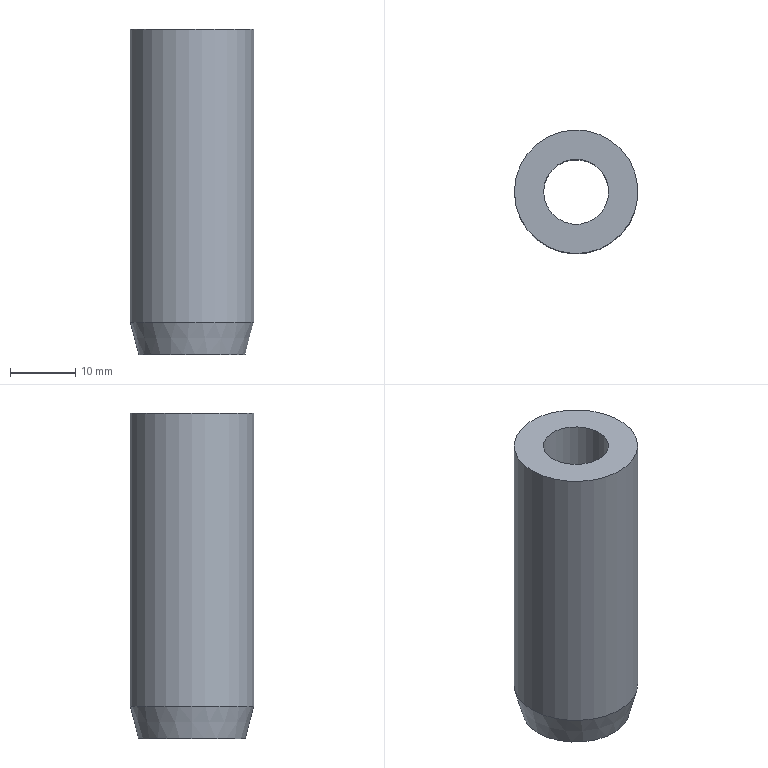Part | NX | features solid 2 | 1 solid | 5 faces | box 19 x 19 x 50 mm | volume 10065 mm3 | plane 2 | cylinder 2 | cone 1 | commonest cylinder face diameters 10 x1 19 x1
STEP:
#1=CARTESIAN_POINT('',(-824.5,-155.,320.));
#2=VERTEX_POINT('',#1);
#3=CARTESIAN_POINT('',(-815.,-155.,320.));
#4=DIRECTION('',(0.,0.,-1.));
#5=DIRECTION('',(-1.,0.,0.));
#6=AXIS2_PLACEMENT_3D('',#3,#4,#5);
#7=CIRCLE('',#6,9.5);
#8=EDGE_CURVE('',#2,#2,#7,.T.);
#9=ORIENTED_EDGE('',*,*,#8,.F.);
#10=EDGE_LOOP('',(#9));
#11=FACE_BOUND('',#10,.T.);
#12=CARTESIAN_POINT('',(-820.,-155.,320.));
#13=VERTEX_POINT('',#12);
#14=CARTESIAN_POINT('',(-815.,-155.,320.));
#15=DIRECTION('',(0.,0.,-1.));
#16=DIRECTION('',(-1.,0.,0.));
#17=AXIS2_PLACEMENT_3D('',#14,#15,#16);
#18=CIRCLE('',#17,5.);
#19=EDGE_CURVE('',#13,#13,#18,.T.);
#20=ORIENTED_EDGE('',*,*,#19,.T.);
#21=EDGE_LOOP('',(#20));
#22=FACE_BOUND('',#21,.T.);
#23=CARTESIAN_POINT('',(-810.,-155.,320.));
#24=DIRECTION('',(0.,0.,-1.));
#25=DIRECTION('',(-1.,0.,0.));
#26=AXIS2_PLACEMENT_3D('',#23,#24,#25);
#27=PLANE('',#26);
#28=ADVANCED_FACE('',(#11,#22),#27,.F.);
#29=CARTESIAN_POINT('',(-824.5,-155.,275.));
#30=VERTEX_POINT('',#29);
#31=CARTESIAN_POINT('',(-815.,-155.,275.));
#32=DIRECTION('',(0.,0.,-1.));
#33=DIRECTION('',(-1.,0.,0.));
#34=AXIS2_PLACEMENT_3D('',#31,#32,#33);
#35=CIRCLE('',#34,9.5);
#36=EDGE_CURVE('',#30,#30,#35,.T.);
#37=ORIENTED_EDGE('',*,*,#36,.F.);
#38=EDGE_LOOP('',(#37));
#39=FACE_BOUND('',#38,.T.);
#40=ORIENTED_EDGE('',*,*,#8,.T.);
#41=EDGE_LOOP('',(#40));
#42=FACE_BOUND('',#41,.T.);
#43=CARTESIAN_POINT('',(-815.,-155.,325.));
#44=DIRECTION('',(0.,0.,-1.));
#45=DIRECTION('',(-1.,0.,0.));
#46=AXIS2_PLACEMENT_3D('',#43,#44,#45);
#47=CYLINDRICAL_SURFACE('',#46,9.5);
#48=ADVANCED_FACE('',(#39,#42),#47,.T.);
#49=CARTESIAN_POINT('',(-823.206,-155.,270.));
#50=VERTEX_POINT('',#49);
#51=CARTESIAN_POINT('',(-815.,-155.,270.));
#52=DIRECTION('',(0.,0.,-1.));
#53=DIRECTION('',(-1.,0.,0.));
#54=AXIS2_PLACEMENT_3D('',#51,#52,#53);
#55=CIRCLE('',#54,8.206);
#56=EDGE_CURVE('',#50,#50,#55,.T.);
#57=ORIENTED_EDGE('',*,*,#56,.F.);
#58=EDGE_LOOP('',(#57));
#59=FACE_BOUND('',#58,.T.);
#60=ORIENTED_EDGE('',*,*,#36,.T.);
#61=EDGE_LOOP('',(#60));
#62=FACE_BOUND('',#61,.T.);
#63=CARTESIAN_POINT('',(-815.,-155.,275.));
#64=DIRECTION('',(0.,0.,1.));
#65=DIRECTION('',(1.,0.,0.));
#66=AXIS2_PLACEMENT_3D('',#63,#64,#65);
#67=CONICAL_SURFACE('',#66,9.5,0.2533);
#68=ADVANCED_FACE('',(#59,#62),#67,.T.);
#69=CARTESIAN_POINT('',(-820.,-155.,270.));
#70=VERTEX_POINT('',#69);
#71=CARTESIAN_POINT('',(-815.,-155.,270.));
#72=DIRECTION('',(0.,0.,-1.));
#73=DIRECTION('',(-1.,0.,0.));
#74=AXIS2_PLACEMENT_3D('',#71,#72,#73);
#75=CIRCLE('',#74,5.);
#76=EDGE_CURVE('',#70,#70,#75,.T.);
#77=ORIENTED_EDGE('',*,*,#76,.F.);
#78=EDGE_LOOP('',(#77));
#79=FACE_BOUND('',#78,.T.);
#80=ORIENTED_EDGE('',*,*,#56,.T.);
#81=EDGE_LOOP('',(#80));
#82=FACE_BOUND('',#81,.T.);
#83=CARTESIAN_POINT('',(-806.794,-155.,270.));
#84=DIRECTION('',(0.,0.,1.));
#85=DIRECTION('',(1.,0.,0.));
#86=AXIS2_PLACEMENT_3D('',#83,#84,#85);
#87=PLANE('',#86);
#88=ADVANCED_FACE('',(#79,#82),#87,.F.);
#89=ORIENTED_EDGE('',*,*,#19,.F.);
#90=EDGE_LOOP('',(#89));
#91=FACE_BOUND('',#90,.T.);
#92=ORIENTED_EDGE('',*,*,#76,.T.);
#93=EDGE_LOOP('',(#92));
#94=FACE_BOUND('',#93,.T.);
#95=CARTESIAN_POINT('',(-815.,-155.,325.));
#96=DIRECTION('',(0.,0.,-1.));
#97=DIRECTION('',(-1.,0.,0.));
#98=AXIS2_PLACEMENT_3D('',#95,#96,#97);
#99=CYLINDRICAL_SURFACE('',#98,5.);
#100=ADVANCED_FACE('',(#91,#94),#99,.F.);
#101=CLOSED_SHELL('',(#28,#48,#68,#88,#100));
#102=MANIFOLD_SOLID_BREP('',#101);
#103=(LENGTH_UNIT()NAMED_UNIT(*)SI_UNIT(.MILLI.,.METRE.));
#104=UNCERTAINTY_MEASURE_WITH_UNIT(LENGTH_MEASURE(0.00001),#103,'','');
#105=(NAMED_UNIT(*)PLANE_ANGLE_UNIT()SI_UNIT($,.RADIAN.));
#106=(NAMED_UNIT(*)SI_UNIT($,.STERADIAN.)SOLID_ANGLE_UNIT());
#107=(GEOMETRIC_REPRESENTATION_CONTEXT(3)GLOBAL_UNCERTAINTY_ASSIGNED_CONTEXT((#104))GLOBAL_UNIT_ASSIGNED_CONTEXT((#103,#105,#106))REPRESENTATION_CONTEXT('',''));
#108=ADVANCED_BREP_SHAPE_REPRESENTATION('',(#102),#107);